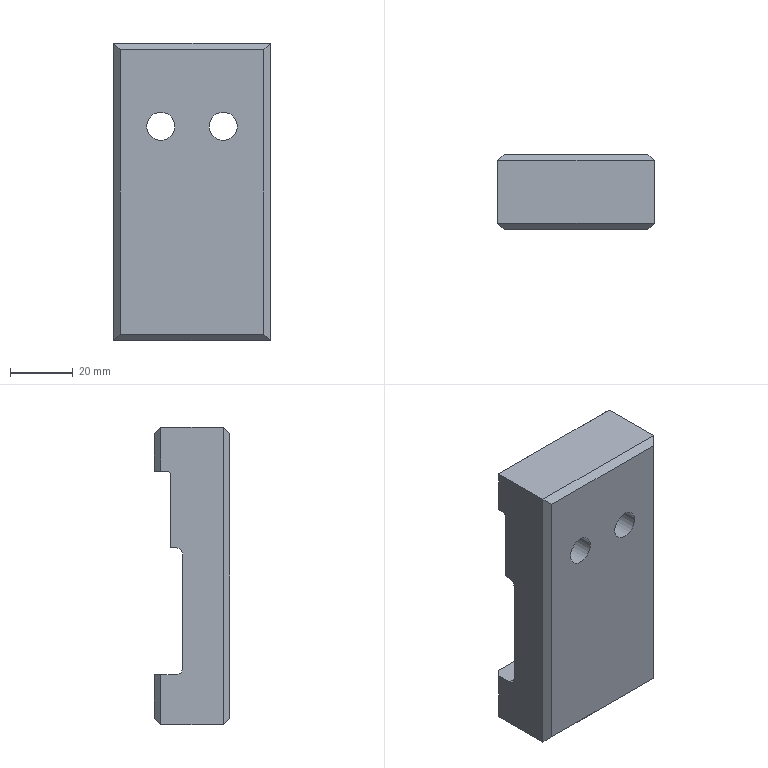Part | NX | features UB-3 2 | 1 solid | 27 faces | box 50 x 24 x 95 mm | volume 86447 mm3 | plane 22 | cylinder 5 | commonest cylinder face diameters 4 x2 9.007 x2 2 x1
STEP:
#1=CARTESIAN_POINT('',(3443.094,-993.122,945.716));
#2=VERTEX_POINT('',#1);
#3=CARTESIAN_POINT('',(3397.094,-993.122,945.716));
#4=VERTEX_POINT('',#3);
#5=CARTESIAN_POINT('',(3420.094,-993.122,945.716));
#6=DIRECTION('',(-1.,0.,0.));
#7=VECTOR('',#6,1000.);
#8=LINE('',#5,#7);
#9=EDGE_CURVE('',#2,#4,#8,.T.);
#10=ORIENTED_EDGE('',*,*,#9,.F.);
#11=CARTESIAN_POINT('',(3445.094,-995.122,945.716));
#12=VERTEX_POINT('',#11);
#13=CARTESIAN_POINT('',(3437.594,-987.622,945.716));
#14=DIRECTION('',(0.7071,-0.7071,0.));
#15=VECTOR('',#14,1000.);
#16=LINE('',#13,#15);
#17=EDGE_CURVE('',#2,#12,#16,.T.);
#18=ORIENTED_EDGE('',*,*,#17,.T.);
#19=CARTESIAN_POINT('',(3445.094,-997.122,945.716));
#20=VERTEX_POINT('',#19);
#21=CARTESIAN_POINT('',(3445.094,-1012.122,945.716));
#22=DIRECTION('',(0.,1.,0.));
#23=VECTOR('',#22,1000.);
#24=LINE('',#21,#23);
#25=EDGE_CURVE('',#20,#12,#24,.T.);
#26=ORIENTED_EDGE('',*,*,#25,.F.);
#27=CARTESIAN_POINT('',(3395.094,-997.122,945.716));
#28=VERTEX_POINT('',#27);
#29=CARTESIAN_POINT('',(3420.094,-997.122,945.716));
#30=DIRECTION('',(-1.,0.,0.));
#31=VECTOR('',#30,1000.);
#32=LINE('',#29,#31);
#33=EDGE_CURVE('',#20,#28,#32,.T.);
#34=ORIENTED_EDGE('',*,*,#33,.T.);
#35=CARTESIAN_POINT('',(3395.094,-995.122,945.716));
#36=VERTEX_POINT('',#35);
#37=CARTESIAN_POINT('',(3395.094,-802.122,945.716));
#38=DIRECTION('',(0.,1.,0.));
#39=VECTOR('',#38,1000.);
#40=LINE('',#37,#39);
#41=EDGE_CURVE('',#28,#36,#40,.T.);
#42=ORIENTED_EDGE('',*,*,#41,.T.);
#43=CARTESIAN_POINT('',(3402.594,-987.622,945.716));
#44=DIRECTION('',(0.7071,0.7071,0.));
#45=VECTOR('',#44,1000.);
#46=LINE('',#43,#45);
#47=EDGE_CURVE('',#36,#4,#46,.T.);
#48=ORIENTED_EDGE('',*,*,#47,.T.);
#49=EDGE_LOOP('',(#10,#18,#26,#34,#42,#48));
#50=FACE_BOUND('',#49,.T.);
#51=CARTESIAN_POINT('',(3420.094,-1005.122,945.716));
#52=DIRECTION('',(0.,0.,-1.));
#53=DIRECTION('',(-1.,0.,0.));
#54=AXIS2_PLACEMENT_3D('',#51,#52,#53);
#55=PLANE('',#54);
#56=ADVANCED_FACE('',(#50),#55,.T.);
#57=CARTESIAN_POINT('',(3395.094,-995.122,959.716));
#58=VERTEX_POINT('',#57);
#59=CARTESIAN_POINT('',(3395.094,-1015.122,959.716));
#60=VERTEX_POINT('',#59);
#61=CARTESIAN_POINT('',(3395.094,-1012.122,959.716));
#62=DIRECTION('',(0.,-1.,0.));
#63=VECTOR('',#62,1000.);
#64=LINE('',#61,#63);
#65=EDGE_CURVE('',#58,#60,#64,.T.);
#66=ORIENTED_EDGE('',*,*,#65,.T.);
#67=CARTESIAN_POINT('',(3445.094,-1015.122,959.716));
#68=VERTEX_POINT('',#67);
#69=CARTESIAN_POINT('',(3140.094,-1015.122,959.716));
#70=DIRECTION('',(1.,0.,0.));
#71=VECTOR('',#70,1000.);
#72=LINE('',#69,#71);
#73=EDGE_CURVE('',#60,#68,#72,.T.);
#74=ORIENTED_EDGE('',*,*,#73,.T.);
#75=CARTESIAN_POINT('',(3445.094,-995.122,959.716));
#76=VERTEX_POINT('',#75);
#77=CARTESIAN_POINT('',(3445.094,-1012.122,959.716));
#78=DIRECTION('',(0.,-1.,0.));
#79=VECTOR('',#78,1000.);
#80=LINE('',#77,#79);
#81=EDGE_CURVE('',#76,#68,#80,.T.);
#82=ORIENTED_EDGE('',*,*,#81,.F.);
#83=CARTESIAN_POINT('',(3140.094,-995.122,959.716));
#84=DIRECTION('',(-1.,0.,0.));
#85=VECTOR('',#84,1000.);
#86=LINE('',#83,#85);
#87=EDGE_CURVE('',#76,#58,#86,.T.);
#88=ORIENTED_EDGE('',*,*,#87,.T.);
#89=EDGE_LOOP('',(#66,#74,#82,#88));
#90=FACE_BOUND('',#89,.T.);
#91=CARTESIAN_POINT('',(3140.094,-1012.122,959.716));
#92=DIRECTION('',(0.,0.,1.));
#93=DIRECTION('',(1.,0.,0.));
#94=AXIS2_PLACEMENT_3D('',#91,#92,#93);
#95=PLANE('',#94);
#96=ADVANCED_FACE('',(#90),#95,.T.);
#97=CARTESIAN_POINT('',(3397.094,-993.122,957.716));
#98=VERTEX_POINT('',#97);
#99=CARTESIAN_POINT('',(3443.094,-993.122,957.716));
#100=VERTEX_POINT('',#99);
#101=CARTESIAN_POINT('',(3420.094,-993.122,957.716));
#102=DIRECTION('',(1.,0.,0.));
#103=VECTOR('',#102,1000.);
#104=LINE('',#101,#103);
#105=EDGE_CURVE('',#98,#100,#104,.T.);
#106=ORIENTED_EDGE('',*,*,#105,.T.);
#107=CARTESIAN_POINT('',(3443.094,-993.122,961.716));
#108=DIRECTION('',(0.,0.,-1.));
#109=VECTOR('',#108,1000.);
#110=LINE('',#107,#109);
#111=EDGE_CURVE('',#100,#2,#110,.T.);
#112=ORIENTED_EDGE('',*,*,#111,.T.);
#113=ORIENTED_EDGE('',*,*,#9,.T.);
#114=CARTESIAN_POINT('',(3397.094,-993.122,928.716));
#115=DIRECTION('',(0.,0.,1.));
#116=VECTOR('',#115,1000.);
#117=LINE('',#114,#116);
#118=EDGE_CURVE('',#4,#98,#117,.T.);
#119=ORIENTED_EDGE('',*,*,#118,.T.);
#120=EDGE_LOOP('',(#106,#112,#113,#119));
#121=FACE_BOUND('',#120,.T.);
#122=CARTESIAN_POINT('',(3420.094,-993.122,928.716));
#123=DIRECTION('',(0.,1.,0.));
#124=DIRECTION('',(0.,0.,-1.));
#125=AXIS2_PLACEMENT_3D('',#122,#123,#124);
#126=PLANE('',#125);
#127=ADVANCED_FACE('',(#121),#126,.T.);
#128=CARTESIAN_POINT('',(3430.094,-1017.122,928.713));
#129=VERTEX_POINT('',#128);
#130=CARTESIAN_POINT('',(3430.094,-1017.122,933.216));
#131=DIRECTION('',(0.,-1.,0.));
#132=DIRECTION('',(0.,0.,-1.));
#133=AXIS2_PLACEMENT_3D('',#130,#131,#132);
#134=CIRCLE('',#133,4.503);
#135=EDGE_CURVE('',#129,#129,#134,.T.);
#136=ORIENTED_EDGE('',*,*,#135,.F.);
#137=EDGE_LOOP('',(#136));
#138=FACE_BOUND('',#137,.T.);
#139=CARTESIAN_POINT('',(3410.094,-1017.122,928.713));
#140=VERTEX_POINT('',#139);
#141=CARTESIAN_POINT('',(3410.094,-1017.122,933.216));
#142=DIRECTION('',(0.,-1.,0.));
#143=DIRECTION('',(0.,0.,-1.));
#144=AXIS2_PLACEMENT_3D('',#141,#142,#143);
#145=CIRCLE('',#144,4.503);
#146=EDGE_CURVE('',#140,#140,#145,.T.);
#147=ORIENTED_EDGE('',*,*,#146,.F.);
#148=EDGE_LOOP('',(#147));
#149=FACE_BOUND('',#148,.T.);
#150=CARTESIAN_POINT('',(3397.094,-1017.122,866.716));
#151=VERTEX_POINT('',#150);
#152=CARTESIAN_POINT('',(3443.094,-1017.122,866.716));
#153=VERTEX_POINT('',#152);
#154=CARTESIAN_POINT('',(3140.094,-1017.122,866.716));
#155=DIRECTION('',(1.,0.,0.));
#156=VECTOR('',#155,1000.);
#157=LINE('',#154,#156);
#158=EDGE_CURVE('',#151,#153,#157,.T.);
#159=ORIENTED_EDGE('',*,*,#158,.T.);
#160=CARTESIAN_POINT('',(3443.094,-1017.122,957.716));
#161=VERTEX_POINT('',#160);
#162=CARTESIAN_POINT('',(3443.094,-1017.122,865.716));
#163=DIRECTION('',(0.,0.,1.));
#164=VECTOR('',#163,1000.);
#165=LINE('',#162,#164);
#166=EDGE_CURVE('',#153,#161,#165,.T.);
#167=ORIENTED_EDGE('',*,*,#166,.T.);
#168=CARTESIAN_POINT('',(3397.094,-1017.122,957.716));
#169=VERTEX_POINT('',#168);
#170=CARTESIAN_POINT('',(3140.094,-1017.122,957.716));
#171=DIRECTION('',(-1.,0.,0.));
#172=VECTOR('',#171,1000.);
#173=LINE('',#170,#172);
#174=EDGE_CURVE('',#161,#169,#173,.T.);
#175=ORIENTED_EDGE('',*,*,#174,.T.);
#176=CARTESIAN_POINT('',(3397.094,-1017.122,858.716));
#177=DIRECTION('',(0.,0.,-1.));
#178=VECTOR('',#177,1000.);
#179=LINE('',#176,#178);
#180=EDGE_CURVE('',#169,#151,#179,.T.);
#181=ORIENTED_EDGE('',*,*,#180,.T.);
#182=EDGE_LOOP('',(#159,#167,#175,#181));
#183=FACE_BOUND('',#182,.T.);
#184=CARTESIAN_POINT('',(3140.094,-1017.122,858.716));
#185=DIRECTION('',(0.,-1.,0.));
#186=DIRECTION('',(0.,0.,1.));
#187=AXIS2_PLACEMENT_3D('',#184,#185,#186);
#188=PLANE('',#187);
#189=ADVANCED_FACE('',(#138,#149,#183),#188,.T.);
#190=CARTESIAN_POINT('',(3445.094,-1000.122,880.716));
#191=VERTEX_POINT('',#190);
#192=CARTESIAN_POINT('',(3445.094,-995.122,880.716));
#193=VERTEX_POINT('',#192);
#194=CARTESIAN_POINT('',(3445.094,-1012.122,880.716));
#195=DIRECTION('',(0.,1.,0.));
#196=VECTOR('',#195,1000.);
#197=LINE('',#194,#196);
#198=EDGE_CURVE('',#191,#193,#197,.T.);
#199=ORIENTED_EDGE('',*,*,#198,.F.);
#200=CARTESIAN_POINT('',(3445.094,-1002.122,882.716));
#201=VERTEX_POINT('',#200);
#202=CARTESIAN_POINT('',(3445.094,-1000.122,882.716));
#203=DIRECTION('',(-1.,0.,0.));
#204=DIRECTION('',(0.,0.,-1.));
#205=AXIS2_PLACEMENT_3D('',#202,#203,#204);
#206=CIRCLE('',#205,2.);
#207=EDGE_CURVE('',#191,#201,#206,.T.);
#208=ORIENTED_EDGE('',*,*,#207,.T.);
#209=CARTESIAN_POINT('',(3445.094,-1002.122,919.216));
#210=VERTEX_POINT('',#209);
#211=CARTESIAN_POINT('',(3445.094,-1002.122,858.716));
#212=DIRECTION('',(0.,0.,-1.));
#213=VECTOR('',#212,1000.);
#214=LINE('',#211,#213);
#215=EDGE_CURVE('',#210,#201,#214,.T.);
#216=ORIENTED_EDGE('',*,*,#215,.F.);
#217=CARTESIAN_POINT('',(3445.094,-1000.122,921.216));
#218=VERTEX_POINT('',#217);
#219=CARTESIAN_POINT('',(3445.094,-1000.122,919.216));
#220=DIRECTION('',(-1.,0.,0.));
#221=DIRECTION('',(0.,0.,-1.));
#222=AXIS2_PLACEMENT_3D('',#219,#220,#221);
#223=CIRCLE('',#222,2.);
#224=EDGE_CURVE('',#210,#218,#223,.T.);
#225=ORIENTED_EDGE('',*,*,#224,.T.);
#226=CARTESIAN_POINT('',(3445.094,-998.122,921.216));
#227=VERTEX_POINT('',#226);
#228=CARTESIAN_POINT('',(3445.094,-1012.122,921.216));
#229=DIRECTION('',(0.,-1.,0.));
#230=VECTOR('',#229,1000.);
#231=LINE('',#228,#230);
#232=EDGE_CURVE('',#227,#218,#231,.T.);
#233=ORIENTED_EDGE('',*,*,#232,.F.);
#234=CARTESIAN_POINT('',(3445.094,-998.122,944.716));
#235=VERTEX_POINT('',#234);
#236=CARTESIAN_POINT('',(3445.094,-998.122,858.716));
#237=DIRECTION('',(0.,0.,1.));
#238=VECTOR('',#237,1000.);
#239=LINE('',#236,#238);
#240=EDGE_CURVE('',#227,#235,#239,.T.);
#241=ORIENTED_EDGE('',*,*,#240,.T.);
#242=CARTESIAN_POINT('',(3445.094,-997.122,944.716));
#243=DIRECTION('',(-1.,0.,0.));
#244=DIRECTION('',(0.,0.,-1.));
#245=AXIS2_PLACEMENT_3D('',#242,#243,#244);
#246=CIRCLE('',#245,1.);
#247=EDGE_CURVE('',#235,#20,#246,.T.);
#248=ORIENTED_EDGE('',*,*,#247,.T.);
#249=ORIENTED_EDGE('',*,*,#25,.T.);
#250=CARTESIAN_POINT('',(3445.094,-995.122,945.716));
#251=DIRECTION('',(0.,0.,1.));
#252=VECTOR('',#251,1000.);
#253=LINE('',#250,#252);
#254=EDGE_CURVE('',#12,#76,#253,.T.);
#255=ORIENTED_EDGE('',*,*,#254,.T.);
#256=ORIENTED_EDGE('',*,*,#81,.T.);
#257=CARTESIAN_POINT('',(3445.094,-1015.122,864.716));
#258=VERTEX_POINT('',#257);
#259=CARTESIAN_POINT('',(3445.094,-1015.122,961.716));
#260=DIRECTION('',(0.,0.,-1.));
#261=VECTOR('',#260,1000.);
#262=LINE('',#259,#261);
#263=EDGE_CURVE('',#68,#258,#262,.T.);
#264=ORIENTED_EDGE('',*,*,#263,.T.);
#265=CARTESIAN_POINT('',(3445.094,-995.122,864.716));
#266=VERTEX_POINT('',#265);
#267=CARTESIAN_POINT('',(3445.094,-1012.122,864.716));
#268=DIRECTION('',(0.,1.,0.));
#269=VECTOR('',#268,1000.);
#270=LINE('',#267,#269);
#271=EDGE_CURVE('',#258,#266,#270,.T.);
#272=ORIENTED_EDGE('',*,*,#271,.T.);
#273=CARTESIAN_POINT('',(3445.094,-995.122,866.716));
#274=DIRECTION('',(0.,0.,1.));
#275=VECTOR('',#274,1000.);
#276=LINE('',#273,#275);
#277=EDGE_CURVE('',#266,#193,#276,.T.);
#278=ORIENTED_EDGE('',*,*,#277,.T.);
#279=EDGE_LOOP('',(#199,#208,#216,#225,#233,#241,#248,#249,#255,#256,#264,#272,#278));
#280=FACE_BOUND('',#279,.T.);
#281=CARTESIAN_POINT('',(3445.094,-1012.122,858.716));
#282=DIRECTION('',(-1.,0.,0.));
#283=DIRECTION('',(0.,0.,-1.));
#284=AXIS2_PLACEMENT_3D('',#281,#282,#283);
#285=PLANE('',#284);
#286=ADVANCED_FACE('',(#280),#285,.F.);
#287=CARTESIAN_POINT('',(3395.094,-1015.122,864.716));
#288=VERTEX_POINT('',#287);
#289=CARTESIAN_POINT('',(3395.094,-995.122,864.716));
#290=VERTEX_POINT('',#289);
#291=CARTESIAN_POINT('',(3395.094,-802.122,864.716));
#292=DIRECTION('',(0.,1.,0.));
#293=VECTOR('',#292,1000.);
#294=LINE('',#291,#293);
#295=EDGE_CURVE('',#288,#290,#294,.T.);
#296=ORIENTED_EDGE('',*,*,#295,.F.);
#297=CARTESIAN_POINT('',(3395.094,-1015.122,928.716));
#298=DIRECTION('',(0.,0.,1.));
#299=VECTOR('',#298,1000.);
#300=LINE('',#297,#299);
#301=EDGE_CURVE('',#288,#60,#300,.T.);
#302=ORIENTED_EDGE('',*,*,#301,.T.);
#303=ORIENTED_EDGE('',*,*,#65,.F.);
#304=CARTESIAN_POINT('',(3395.094,-995.122,928.716));
#305=DIRECTION('',(0.,0.,-1.));
#306=VECTOR('',#305,1000.);
#307=LINE('',#304,#306);
#308=EDGE_CURVE('',#58,#36,#307,.T.);
#309=ORIENTED_EDGE('',*,*,#308,.T.);
#310=ORIENTED_EDGE('',*,*,#41,.F.);
#311=CARTESIAN_POINT('',(3395.094,-998.122,944.716));
#312=VERTEX_POINT('',#311);
#313=CARTESIAN_POINT('',(3395.094,-997.122,944.716));
#314=DIRECTION('',(1.,0.,0.));
#315=DIRECTION('',(0.,0.,-1.));
#316=AXIS2_PLACEMENT_3D('',#313,#314,#315);
#317=CIRCLE('',#316,1.);
#318=EDGE_CURVE('',#28,#312,#317,.T.);
#319=ORIENTED_EDGE('',*,*,#318,.T.);
#320=CARTESIAN_POINT('',(3395.094,-998.122,921.216));
#321=VERTEX_POINT('',#320);
#322=CARTESIAN_POINT('',(3395.094,-998.122,928.716));
#323=DIRECTION('',(0.,0.,1.));
#324=VECTOR('',#323,1000.);
#325=LINE('',#322,#324);
#326=EDGE_CURVE('',#321,#312,#325,.T.);
#327=ORIENTED_EDGE('',*,*,#326,.F.);
#328=CARTESIAN_POINT('',(3395.094,-1000.122,921.216));
#329=VERTEX_POINT('',#328);
#330=CARTESIAN_POINT('',(3395.094,-802.122,921.216));
#331=DIRECTION('',(0.,-1.,0.));
#332=VECTOR('',#331,1000.);
#333=LINE('',#330,#332);
#334=EDGE_CURVE('',#321,#329,#333,.T.);
#335=ORIENTED_EDGE('',*,*,#334,.T.);
#336=CARTESIAN_POINT('',(3395.094,-1002.122,919.216));
#337=VERTEX_POINT('',#336);
#338=CARTESIAN_POINT('',(3395.094,-1000.122,919.216));
#339=DIRECTION('',(1.,0.,0.));
#340=DIRECTION('',(0.,0.,-1.));
#341=AXIS2_PLACEMENT_3D('',#338,#339,#340);
#342=CIRCLE('',#341,2.);
#343=EDGE_CURVE('',#329,#337,#342,.T.);
#344=ORIENTED_EDGE('',*,*,#343,.T.);
#345=CARTESIAN_POINT('',(3395.094,-1002.122,882.716));
#346=VERTEX_POINT('',#345);
#347=CARTESIAN_POINT('',(3395.094,-1002.122,928.716));
#348=DIRECTION('',(0.,0.,1.));
#349=VECTOR('',#348,1000.);
#350=LINE('',#347,#349);
#351=EDGE_CURVE('',#346,#337,#350,.T.);
#352=ORIENTED_EDGE('',*,*,#351,.F.);
#353=CARTESIAN_POINT('',(3395.094,-1000.122,880.716));
#354=VERTEX_POINT('',#353);
#355=CARTESIAN_POINT('',(3395.094,-1000.122,882.716));
#356=DIRECTION('',(1.,0.,0.));
#357=DIRECTION('',(0.,0.,-1.));
#358=AXIS2_PLACEMENT_3D('',#355,#356,#357);
#359=CIRCLE('',#358,2.);
#360=EDGE_CURVE('',#346,#354,#359,.T.);
#361=ORIENTED_EDGE('',*,*,#360,.T.);
#362=CARTESIAN_POINT('',(3395.094,-995.122,880.716));
#363=VERTEX_POINT('',#362);
#364=CARTESIAN_POINT('',(3395.094,-802.122,880.716));
#365=DIRECTION('',(0.,1.,0.));
#366=VECTOR('',#365,1000.);
#367=LINE('',#364,#366);
#368=EDGE_CURVE('',#354,#363,#367,.T.);
#369=ORIENTED_EDGE('',*,*,#368,.T.);
#370=CARTESIAN_POINT('',(3395.094,-995.122,929.716));
#371=DIRECTION('',(0.,0.,-1.));
#372=VECTOR('',#371,1000.);
#373=LINE('',#370,#372);
#374=EDGE_CURVE('',#363,#290,#373,.T.);
#375=ORIENTED_EDGE('',*,*,#374,.T.);
#376=EDGE_LOOP('',(#296,#302,#303,#309,#310,#319,#327,#335,#344,#352,#361,#369,#375));
#377=FACE_BOUND('',#376,.T.);
#378=CARTESIAN_POINT('',(3395.094,-802.122,928.716));
#379=DIRECTION('',(-1.,0.,0.));
#380=DIRECTION('',(0.,0.,1.));
#381=AXIS2_PLACEMENT_3D('',#378,#379,#380);
#382=PLANE('',#381);
#383=ADVANCED_FACE('',(#377),#382,.T.);
#384=ORIENTED_EDGE('',*,*,#351,.T.);
#385=CARTESIAN_POINT('',(3420.094,-1002.122,919.216));
#386=DIRECTION('',(1.,0.,0.));
#387=VECTOR('',#386,1000.);
#388=LINE('',#385,#387);
#389=EDGE_CURVE('',#337,#210,#388,.T.);
#390=ORIENTED_EDGE('',*,*,#389,.T.);
#391=ORIENTED_EDGE('',*,*,#215,.T.);
#392=CARTESIAN_POINT('',(3445.094,-1002.122,882.716));
#393=DIRECTION('',(-1.,0.,0.));
#394=VECTOR('',#393,1000.);
#395=LINE('',#392,#394);
#396=EDGE_CURVE('',#201,#346,#395,.T.);
#397=ORIENTED_EDGE('',*,*,#396,.T.);
#398=EDGE_LOOP('',(#384,#390,#391,#397));
#399=FACE_BOUND('',#398,.T.);
#400=CARTESIAN_POINT('',(3420.094,-1002.122,954.716));
#401=DIRECTION('',(0.,-1.,0.));
#402=DIRECTION('',(0.,0.,1.));
#403=AXIS2_PLACEMENT_3D('',#400,#401,#402);
#404=PLANE('',#403);
#405=ADVANCED_FACE('',(#399),#404,.F.);
#406=ORIENTED_EDGE('',*,*,#295,.T.);
#407=CARTESIAN_POINT('',(3420.094,-995.122,864.716));
#408=DIRECTION('',(1.,0.,0.));
#409=VECTOR('',#408,1000.);
#410=LINE('',#407,#409);
#411=EDGE_CURVE('',#290,#266,#410,.T.);
#412=ORIENTED_EDGE('',*,*,#411,.T.);
#413=ORIENTED_EDGE('',*,*,#271,.F.);
#414=CARTESIAN_POINT('',(3420.094,-1015.122,864.716));
#415=DIRECTION('',(-1.,0.,0.));
#416=VECTOR('',#415,1000.);
#417=LINE('',#414,#416);
#418=EDGE_CURVE('',#258,#288,#417,.T.);
#419=ORIENTED_EDGE('',*,*,#418,.T.);
#420=EDGE_LOOP('',(#406,#412,#413,#419));
#421=FACE_BOUND('',#420,.T.);
#422=CARTESIAN_POINT('',(3420.094,-1005.122,864.716));
#423=DIRECTION('',(0.,0.,-1.));
#424=DIRECTION('',(-1.,0.,0.));
#425=AXIS2_PLACEMENT_3D('',#422,#423,#424);
#426=PLANE('',#425);
#427=ADVANCED_FACE('',(#421),#426,.T.);
#428=CARTESIAN_POINT('',(3430.094,-998.122,928.713));
#429=VERTEX_POINT('',#428);
#430=CARTESIAN_POINT('',(3430.094,-998.122,933.216));
#431=DIRECTION('',(0.,-1.,0.));
#432=DIRECTION('',(0.,0.,-1.));
#433=AXIS2_PLACEMENT_3D('',#430,#431,#432);
#434=CIRCLE('',#433,4.503);
#435=EDGE_CURVE('',#429,#429,#434,.T.);
#436=ORIENTED_EDGE('',*,*,#435,.T.);
#437=EDGE_LOOP('',(#436));
#438=FACE_BOUND('',#437,.T.);
#439=CARTESIAN_POINT('',(3410.094,-998.122,928.713));
#440=VERTEX_POINT('',#439);
#441=CARTESIAN_POINT('',(3410.094,-998.122,933.216));
#442=DIRECTION('',(0.,-1.,0.));
#443=DIRECTION('',(0.,0.,-1.));
#444=AXIS2_PLACEMENT_3D('',#441,#442,#443);
#445=CIRCLE('',#444,4.503);
#446=EDGE_CURVE('',#440,#440,#445,.T.);
#447=ORIENTED_EDGE('',*,*,#446,.T.);
#448=EDGE_LOOP('',(#447));
#449=FACE_BOUND('',#448,.T.);
#450=ORIENTED_EDGE('',*,*,#240,.F.);
#451=CARTESIAN_POINT('',(3420.094,-998.122,921.216));
#452=DIRECTION('',(-1.,0.,0.));
#453=VECTOR('',#452,1000.);
#454=LINE('',#451,#453);
#455=EDGE_CURVE('',#227,#321,#454,.T.);
#456=ORIENTED_EDGE('',*,*,#455,.T.);
#457=ORIENTED_EDGE('',*,*,#326,.T.);
#458=CARTESIAN_POINT('',(3420.094,-998.122,944.716));
#459=DIRECTION('',(1.,0.,0.));
#460=VECTOR('',#459,1000.);
#461=LINE('',#458,#460);
#462=EDGE_CURVE('',#312,#235,#461,.T.);
#463=ORIENTED_EDGE('',*,*,#462,.T.);
#464=EDGE_LOOP('',(#450,#456,#457,#463));
#465=FACE_BOUND('',#464,.T.);
#466=CARTESIAN_POINT('',(3420.094,-998.122,919.716));
#467=DIRECTION('',(0.,-1.,0.));
#468=DIRECTION('',(0.,0.,1.));
#469=AXIS2_PLACEMENT_3D('',#466,#467,#468);
#470=PLANE('',#469);
#471=ADVANCED_FACE('',(#438,#449,#465),#470,.F.);
#472=ORIENTED_EDGE('',*,*,#334,.F.);
#473=ORIENTED_EDGE('',*,*,#455,.F.);
#474=ORIENTED_EDGE('',*,*,#232,.T.);
#475=CARTESIAN_POINT('',(3420.094,-1000.122,921.216));
#476=DIRECTION('',(-1.,0.,0.));
#477=VECTOR('',#476,1000.);
#478=LINE('',#475,#477);
#479=EDGE_CURVE('',#218,#329,#478,.T.);
#480=ORIENTED_EDGE('',*,*,#479,.T.);
#481=EDGE_LOOP('',(#472,#473,#474,#480));
#482=FACE_BOUND('',#481,.T.);
#483=CARTESIAN_POINT('',(3420.094,-1005.122,921.216));
#484=DIRECTION('',(0.,0.,-1.));
#485=DIRECTION('',(-1.,0.,0.));
#486=AXIS2_PLACEMENT_3D('',#483,#484,#485);
#487=PLANE('',#486);
#488=ADVANCED_FACE('',(#482),#487,.T.);
#489=ORIENTED_EDGE('',*,*,#368,.F.);
#490=CARTESIAN_POINT('',(3395.094,-1000.122,880.716));
#491=DIRECTION('',(1.,0.,0.));
#492=VECTOR('',#491,1000.);
#493=LINE('',#490,#492);
#494=EDGE_CURVE('',#354,#191,#493,.T.);
#495=ORIENTED_EDGE('',*,*,#494,.T.);
#496=ORIENTED_EDGE('',*,*,#198,.T.);
#497=CARTESIAN_POINT('',(3443.094,-993.122,880.716));
#498=VERTEX_POINT('',#497);
#499=CARTESIAN_POINT('',(3443.094,-993.122,880.716));
#500=DIRECTION('',(-0.7071,0.7071,0.));
#501=VECTOR('',#500,1000.);
#502=LINE('',#499,#501);
#503=EDGE_CURVE('',#193,#498,#502,.T.);
#504=ORIENTED_EDGE('',*,*,#503,.T.);
#505=CARTESIAN_POINT('',(3397.094,-993.122,880.716));
#506=VERTEX_POINT('',#505);
#507=CARTESIAN_POINT('',(3420.094,-993.122,880.716));
#508=DIRECTION('',(1.,0.,0.));
#509=VECTOR('',#508,1000.);
#510=LINE('',#507,#509);
#511=EDGE_CURVE('',#506,#498,#510,.T.);
#512=ORIENTED_EDGE('',*,*,#511,.F.);
#513=CARTESIAN_POINT('',(3395.094,-995.122,880.716));
#514=DIRECTION('',(-0.7071,-0.7071,0.));
#515=VECTOR('',#514,1000.);
#516=LINE('',#513,#515);
#517=EDGE_CURVE('',#506,#363,#516,.T.);
#518=ORIENTED_EDGE('',*,*,#517,.T.);
#519=EDGE_LOOP('',(#489,#495,#496,#504,#512,#518));
#520=FACE_BOUND('',#519,.T.);
#521=CARTESIAN_POINT('',(3420.094,-1005.122,880.716));
#522=DIRECTION('',(0.,0.,-1.));
#523=DIRECTION('',(-1.,0.,0.));
#524=AXIS2_PLACEMENT_3D('',#521,#522,#523);
#525=PLANE('',#524);
#526=ADVANCED_FACE('',(#520),#525,.F.);
#527=ORIENTED_EDGE('',*,*,#511,.T.);
#528=CARTESIAN_POINT('',(3443.094,-993.122,866.716));
#529=VERTEX_POINT('',#528);
#530=CARTESIAN_POINT('',(3443.094,-993.122,880.716));
#531=DIRECTION('',(0.,0.,-1.));
#532=VECTOR('',#531,1000.);
#533=LINE('',#530,#532);
#534=EDGE_CURVE('',#498,#529,#533,.T.);
#535=ORIENTED_EDGE('',*,*,#534,.T.);
#536=CARTESIAN_POINT('',(3397.094,-993.122,866.716));
#537=VERTEX_POINT('',#536);
#538=CARTESIAN_POINT('',(3420.094,-993.122,866.716));
#539=DIRECTION('',(-1.,0.,0.));
#540=VECTOR('',#539,1000.);
#541=LINE('',#538,#540);
#542=EDGE_CURVE('',#529,#537,#541,.T.);
#543=ORIENTED_EDGE('',*,*,#542,.T.);
#544=CARTESIAN_POINT('',(3397.094,-993.122,929.716));
#545=DIRECTION('',(0.,0.,1.));
#546=VECTOR('',#545,1000.);
#547=LINE('',#544,#546);
#548=EDGE_CURVE('',#537,#506,#547,.T.);
#549=ORIENTED_EDGE('',*,*,#548,.T.);
#550=EDGE_LOOP('',(#527,#535,#543,#549));
#551=FACE_BOUND('',#550,.T.);
#552=CARTESIAN_POINT('',(3420.094,-993.122,929.716));
#553=DIRECTION('',(0.,1.,0.));
#554=DIRECTION('',(0.,0.,-1.));
#555=AXIS2_PLACEMENT_3D('',#552,#553,#554);
#556=PLANE('',#555);
#557=ADVANCED_FACE('',(#551),#556,.T.);
#558=ORIENTED_EDGE('',*,*,#247,.F.);
#559=ORIENTED_EDGE('',*,*,#462,.F.);
#560=ORIENTED_EDGE('',*,*,#318,.F.);
#561=ORIENTED_EDGE('',*,*,#33,.F.);
#562=EDGE_LOOP('',(#558,#559,#560,#561));
#563=FACE_BOUND('',#562,.T.);
#564=CARTESIAN_POINT('',(3420.094,-997.122,944.716));
#565=DIRECTION('',(-1.,0.,0.));
#566=DIRECTION('',(0.,0.,1.));
#567=AXIS2_PLACEMENT_3D('',#564,#565,#566);
#568=CYLINDRICAL_SURFACE('',#567,1.);
#569=ADVANCED_FACE('',(#563),#568,.F.);
#570=ORIENTED_EDGE('',*,*,#224,.F.);
#571=ORIENTED_EDGE('',*,*,#389,.F.);
#572=ORIENTED_EDGE('',*,*,#343,.F.);
#573=ORIENTED_EDGE('',*,*,#479,.F.);
#574=EDGE_LOOP('',(#570,#571,#572,#573));
#575=FACE_BOUND('',#574,.T.);
#576=CARTESIAN_POINT('',(3420.094,-1000.122,919.216));
#577=DIRECTION('',(-1.,0.,0.));
#578=DIRECTION('',(0.,0.,1.));
#579=AXIS2_PLACEMENT_3D('',#576,#577,#578);
#580=CYLINDRICAL_SURFACE('',#579,2.);
#581=ADVANCED_FACE('',(#575),#580,.F.);
#582=ORIENTED_EDGE('',*,*,#360,.F.);
#583=ORIENTED_EDGE('',*,*,#396,.F.);
#584=ORIENTED_EDGE('',*,*,#207,.F.);
#585=ORIENTED_EDGE('',*,*,#494,.F.);
#586=EDGE_LOOP('',(#582,#583,#584,#585));
#587=FACE_BOUND('',#586,.T.);
#588=CARTESIAN_POINT('',(3420.094,-1000.122,882.716));
#589=DIRECTION('',(-1.,0.,0.));
#590=DIRECTION('',(0.,0.,1.));
#591=AXIS2_PLACEMENT_3D('',#588,#589,#590);
#592=CYLINDRICAL_SURFACE('',#591,2.);
#593=ADVANCED_FACE('',(#587),#592,.F.);
#594=ORIENTED_EDGE('',*,*,#87,.F.);
#595=CARTESIAN_POINT('',(3343.427,-893.455,858.05));
#596=DIRECTION('',(-0.5774,0.5774,-0.5774));
#597=VECTOR('',#596,1000.);
#598=LINE('',#595,#597);
#599=EDGE_CURVE('',#76,#100,#598,.T.);
#600=ORIENTED_EDGE('',*,*,#599,.T.);
#601=ORIENTED_EDGE('',*,*,#105,.F.);
#602=CARTESIAN_POINT('',(3310.094,-1080.122,1044.716));
#603=DIRECTION('',(-0.5774,-0.5774,0.5774));
#604=VECTOR('',#603,1000.);
#605=LINE('',#602,#604);
#606=EDGE_CURVE('',#98,#58,#605,.T.);
#607=ORIENTED_EDGE('',*,*,#606,.T.);
#608=EDGE_LOOP('',(#594,#600,#601,#607));
#609=FACE_BOUND('',#608,.T.);
#610=CARTESIAN_POINT('',(3140.094,-995.122,959.716));
#611=DIRECTION('',(0.,-0.7071,-0.7071));
#612=DIRECTION('',(-1.,0.,0.));
#613=AXIS2_PLACEMENT_3D('',#610,#611,#612);
#614=PLANE('',#613);
#615=ADVANCED_FACE('',(#609),#614,.F.);
#616=ORIENTED_EDGE('',*,*,#174,.F.);
#617=CARTESIAN_POINT('',(3342.094,-1118.122,856.716));
#618=DIRECTION('',(0.5774,0.5774,0.5774));
#619=VECTOR('',#618,1000.);
#620=LINE('',#617,#619);
#621=EDGE_CURVE('',#161,#68,#620,.T.);
#622=ORIENTED_EDGE('',*,*,#621,.T.);
#623=ORIENTED_EDGE('',*,*,#73,.F.);
#624=CARTESIAN_POINT('',(3311.427,-931.455,1043.383));
#625=DIRECTION('',(0.5774,-0.5774,-0.5774));
#626=VECTOR('',#625,1000.);
#627=LINE('',#624,#626);
#628=EDGE_CURVE('',#60,#169,#627,.T.);
#629=ORIENTED_EDGE('',*,*,#628,.T.);
#630=EDGE_LOOP('',(#616,#622,#623,#629));
#631=FACE_BOUND('',#630,.T.);
#632=CARTESIAN_POINT('',(3140.094,-1017.122,957.716));
#633=DIRECTION('',(0.,0.7071,-0.7071));
#634=DIRECTION('',(-1.,0.,0.));
#635=AXIS2_PLACEMENT_3D('',#632,#633,#634);
#636=PLANE('',#635);
#637=ADVANCED_FACE('',(#631),#636,.F.);
#638=ORIENTED_EDGE('',*,*,#418,.F.);
#639=CARTESIAN_POINT('',(3342.094,-1118.122,967.716));
#640=DIRECTION('',(-0.5774,-0.5774,0.5774));
#641=VECTOR('',#640,1000.);
#642=LINE('',#639,#641);
#643=EDGE_CURVE('',#258,#153,#642,.T.);
#644=ORIENTED_EDGE('',*,*,#643,.T.);
#645=ORIENTED_EDGE('',*,*,#158,.F.);
#646=CARTESIAN_POINT('',(3311.427,-931.455,781.05));
#647=DIRECTION('',(-0.5774,0.5774,-0.5774));
#648=VECTOR('',#647,1000.);
#649=LINE('',#646,#648);
#650=EDGE_CURVE('',#151,#288,#649,.T.);
#651=ORIENTED_EDGE('',*,*,#650,.T.);
#652=EDGE_LOOP('',(#638,#644,#645,#651));
#653=FACE_BOUND('',#652,.T.);
#654=CARTESIAN_POINT('',(3140.094,-1017.122,866.716));
#655=DIRECTION('',(0.,0.7071,0.7071));
#656=DIRECTION('',(1.,0.,0.));
#657=AXIS2_PLACEMENT_3D('',#654,#655,#656);
#658=PLANE('',#657);
#659=ADVANCED_FACE('',(#653),#658,.F.);
#660=ORIENTED_EDGE('',*,*,#542,.F.);
#661=CARTESIAN_POINT('',(3435.427,-985.455,874.383));
#662=DIRECTION('',(0.5774,-0.5774,-0.5774));
#663=VECTOR('',#662,1000.);
#664=LINE('',#661,#663);
#665=EDGE_CURVE('',#529,#266,#664,.T.);
#666=ORIENTED_EDGE('',*,*,#665,.T.);
#667=ORIENTED_EDGE('',*,*,#411,.F.);
#668=CARTESIAN_POINT('',(3404.761,-985.455,874.383));
#669=DIRECTION('',(0.5774,0.5774,0.5774));
#670=VECTOR('',#669,1000.);
#671=LINE('',#668,#670);
#672=EDGE_CURVE('',#290,#537,#671,.T.);
#673=ORIENTED_EDGE('',*,*,#672,.T.);
#674=EDGE_LOOP('',(#660,#666,#667,#673));
#675=FACE_BOUND('',#674,.T.);
#676=CARTESIAN_POINT('',(3420.094,-993.122,866.716));
#677=DIRECTION('',(0.,-0.7071,0.7071));
#678=DIRECTION('',(-1.,0.,0.));
#679=AXIS2_PLACEMENT_3D('',#676,#677,#678);
#680=PLANE('',#679);
#681=ADVANCED_FACE('',(#675),#680,.F.);
#682=ORIENTED_EDGE('',*,*,#672,.F.);
#683=ORIENTED_EDGE('',*,*,#374,.F.);
#684=ORIENTED_EDGE('',*,*,#517,.F.);
#685=ORIENTED_EDGE('',*,*,#548,.F.);
#686=EDGE_LOOP('',(#682,#683,#684,#685));
#687=FACE_BOUND('',#686,.T.);
#688=CARTESIAN_POINT('',(3395.094,-995.122,929.716));
#689=DIRECTION('',(0.7071,-0.7071,0.));
#690=DIRECTION('',(0.,0.,-1.));
#691=AXIS2_PLACEMENT_3D('',#688,#689,#690);
#692=PLANE('',#691);
#693=ADVANCED_FACE('',(#687),#692,.F.);
#694=ORIENTED_EDGE('',*,*,#47,.F.);
#695=ORIENTED_EDGE('',*,*,#308,.F.);
#696=ORIENTED_EDGE('',*,*,#606,.F.);
#697=ORIENTED_EDGE('',*,*,#118,.F.);
#698=EDGE_LOOP('',(#694,#695,#696,#697));
#699=FACE_BOUND('',#698,.T.);
#700=CARTESIAN_POINT('',(3395.094,-995.122,928.716));
#701=DIRECTION('',(0.7071,-0.7071,0.));
#702=DIRECTION('',(0.,0.,-1.));
#703=AXIS2_PLACEMENT_3D('',#700,#701,#702);
#704=PLANE('',#703);
#705=ADVANCED_FACE('',(#699),#704,.F.);
#706=ORIENTED_EDGE('',*,*,#665,.F.);
#707=ORIENTED_EDGE('',*,*,#534,.F.);
#708=ORIENTED_EDGE('',*,*,#503,.F.);
#709=ORIENTED_EDGE('',*,*,#277,.F.);
#710=EDGE_LOOP('',(#706,#707,#708,#709));
#711=FACE_BOUND('',#710,.T.);
#712=CARTESIAN_POINT('',(3443.094,-993.122,929.716));
#713=DIRECTION('',(0.7071,0.7071,0.));
#714=DIRECTION('',(0.,0.,1.));
#715=AXIS2_PLACEMENT_3D('',#712,#713,#714);
#716=PLANE('',#715);
#717=ADVANCED_FACE('',(#711),#716,.T.);
#718=ORIENTED_EDGE('',*,*,#17,.F.);
#719=ORIENTED_EDGE('',*,*,#111,.F.);
#720=ORIENTED_EDGE('',*,*,#599,.F.);
#721=ORIENTED_EDGE('',*,*,#254,.F.);
#722=EDGE_LOOP('',(#718,#719,#720,#721));
#723=FACE_BOUND('',#722,.T.);
#724=CARTESIAN_POINT('',(3443.094,-993.122,928.716));
#725=DIRECTION('',(0.7071,0.7071,0.));
#726=DIRECTION('',(0.,0.,1.));
#727=AXIS2_PLACEMENT_3D('',#724,#725,#726);
#728=PLANE('',#727);
#729=ADVANCED_FACE('',(#723),#728,.T.);
#730=ORIENTED_EDGE('',*,*,#650,.F.);
#731=ORIENTED_EDGE('',*,*,#180,.F.);
#732=ORIENTED_EDGE('',*,*,#628,.F.);
#733=ORIENTED_EDGE('',*,*,#301,.F.);
#734=EDGE_LOOP('',(#730,#731,#732,#733));
#735=FACE_BOUND('',#734,.T.);
#736=CARTESIAN_POINT('',(3397.094,-1017.122,858.716));
#737=DIRECTION('',(0.7071,0.7071,0.));
#738=DIRECTION('',(0.,0.,-1.));
#739=AXIS2_PLACEMENT_3D('',#736,#737,#738);
#740=PLANE('',#739);
#741=ADVANCED_FACE('',(#735),#740,.F.);
#742=ORIENTED_EDGE('',*,*,#643,.F.);
#743=ORIENTED_EDGE('',*,*,#263,.F.);
#744=ORIENTED_EDGE('',*,*,#621,.F.);
#745=ORIENTED_EDGE('',*,*,#166,.F.);
#746=EDGE_LOOP('',(#742,#743,#744,#745));
#747=FACE_BOUND('',#746,.T.);
#748=CARTESIAN_POINT('',(3445.094,-1015.122,858.716));
#749=DIRECTION('',(0.7071,-0.7071,0.));
#750=DIRECTION('',(0.,0.,1.));
#751=AXIS2_PLACEMENT_3D('',#748,#749,#750);
#752=PLANE('',#751);
#753=ADVANCED_FACE('',(#747),#752,.T.);
#754=ORIENTED_EDGE('',*,*,#146,.T.);
#755=EDGE_LOOP('',(#754));
#756=FACE_BOUND('',#755,.T.);
#757=ORIENTED_EDGE('',*,*,#446,.F.);
#758=EDGE_LOOP('',(#757));
#759=FACE_BOUND('',#758,.T.);
#760=CARTESIAN_POINT('',(3410.094,-1017.122,933.216));
#761=DIRECTION('',(0.,1.,0.));
#762=DIRECTION('',(1.,0.,0.));
#763=AXIS2_PLACEMENT_3D('',#760,#761,#762);
#764=CYLINDRICAL_SURFACE('',#763,4.503);
#765=ADVANCED_FACE('',(#756,#759),#764,.F.);
#766=ORIENTED_EDGE('',*,*,#135,.T.);
#767=EDGE_LOOP('',(#766));
#768=FACE_BOUND('',#767,.T.);
#769=ORIENTED_EDGE('',*,*,#435,.F.);
#770=EDGE_LOOP('',(#769));
#771=FACE_BOUND('',#770,.T.);
#772=CARTESIAN_POINT('',(3430.094,-1017.122,933.216));
#773=DIRECTION('',(0.,1.,0.));
#774=DIRECTION('',(-1.,0.,0.));
#775=AXIS2_PLACEMENT_3D('',#772,#773,#774);
#776=CYLINDRICAL_SURFACE('',#775,4.503);
#777=ADVANCED_FACE('',(#768,#771),#776,.F.);
#778=CLOSED_SHELL('',(#56,#96,#127,#189,#286,#383,#405,#427,#471,#488,#526,#557,#569,#581,#593,#615,#637,#659,#681,#693,#705,#717,#729,#741,#753,#765,#777));
#779=MANIFOLD_SOLID_BREP('',#778);
#780=(LENGTH_UNIT()NAMED_UNIT(*)SI_UNIT(.MILLI.,.METRE.));
#781=UNCERTAINTY_MEASURE_WITH_UNIT(LENGTH_MEASURE(0.00001),#780,'','');
#782=(NAMED_UNIT(*)PLANE_ANGLE_UNIT()SI_UNIT($,.RADIAN.));
#783=(NAMED_UNIT(*)SI_UNIT($,.STERADIAN.)SOLID_ANGLE_UNIT());
#784=(GEOMETRIC_REPRESENTATION_CONTEXT(3)GLOBAL_UNCERTAINTY_ASSIGNED_CONTEXT((#781))GLOBAL_UNIT_ASSIGNED_CONTEXT((#780,#782,#783))REPRESENTATION_CONTEXT('',''));
#785=ADVANCED_BREP_SHAPE_REPRESENTATION('',(#779),#784);